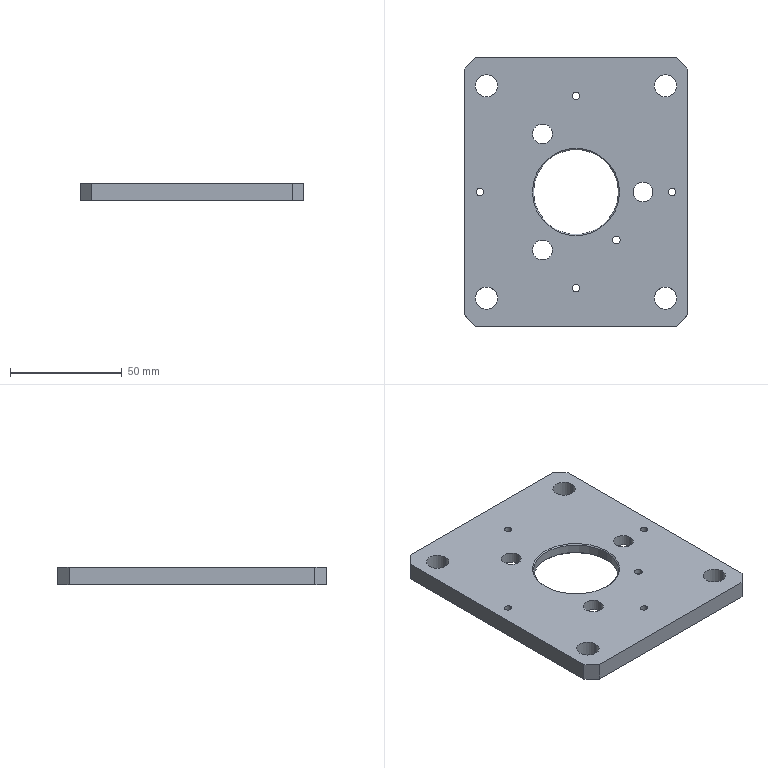Part | STEP file | PN_0030 JIG Plate | 1 solid | 48 faces | box 100 x 120 x 8 mm | volume 64897 mm3 | cylinder 30 | plane 12 | cone 6 | commonest cylinder face diameters 3.3 x8 10 x8 8.8 x6 3.5 x2 6 x2 38 x2